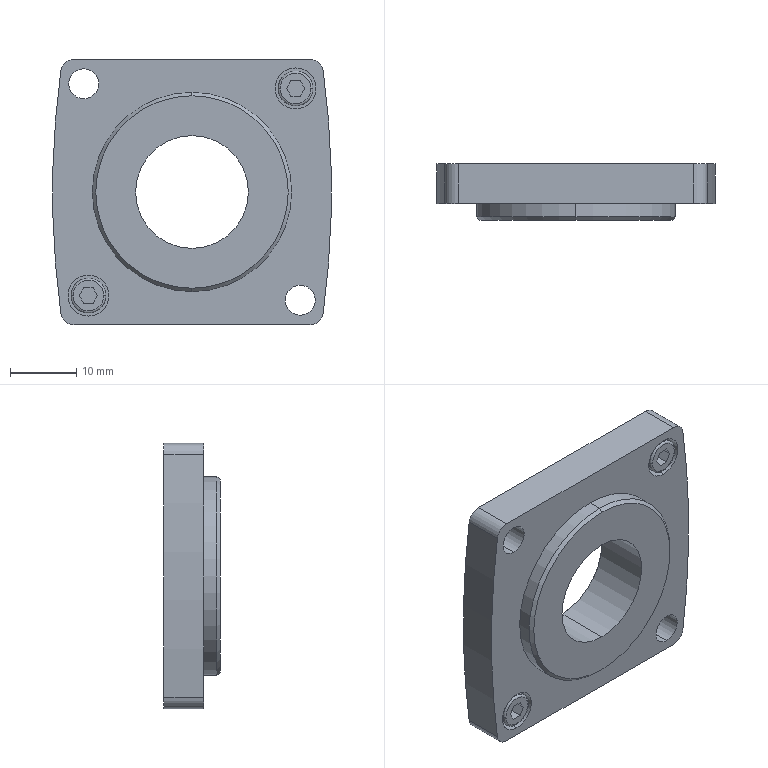Part | SolidWorks | features BaseBody 1 | 1 solid | 80 faces | box 42.009 x 8.51 x 40 mm | volume 9357 mm3 | plane 40 | cylinder 34 | spline 4 | cone 2 | commonest cylinder face diameters 4 x6 3.38 x4 3.4 x4 4.5 x4 5.232 x4 6.18 x4